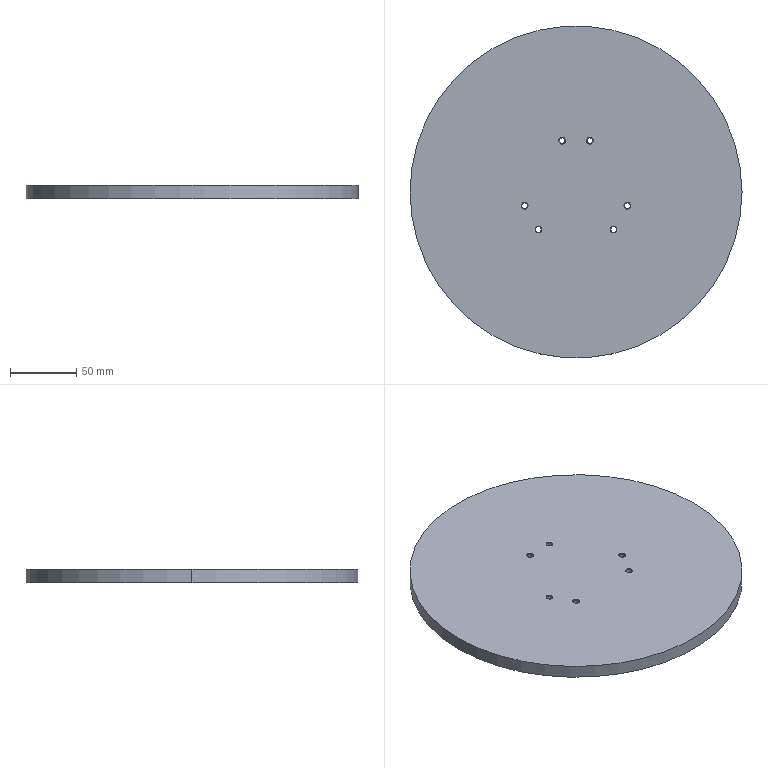Part | SolidWorks | features 3DProfileFeature 1, CirPattern 1, Extrusion 1, HoleWzd 1 | 1 solid | 28 faces | box 250 x 250 x 10 mm | volume 490035 mm3 | cylinder 14 | cone 12 | plane 2 | commonest cylinder face diameters 4.2 x12 250 x2
STEP:
#1=CARTESIAN_POINT('',(26.184,-28.284,9.575));
#2=VERTEX_POINT('',#1);
#3=CARTESIAN_POINT('',(30.384,-28.284,9.575));
#4=VERTEX_POINT('',#3);
#5=CARTESIAN_POINT('',(28.284,-28.284,9.575));
#6=DIRECTION('',(0.,0.,1.));
#7=DIRECTION('',(1.,0.,0.));
#8=AXIS2_PLACEMENT_3D('',#5,#6,#7);
#9=CIRCLE('',#8,2.1);
#10=EDGE_CURVE('',#2,#4,#9,.T.);
#11=ORIENTED_EDGE('',*,*,#10,.F.);
#12=CARTESIAN_POINT('',(25.759,-28.284,10.));
#13=VERTEX_POINT('',#12);
#14=CARTESIAN_POINT('',(25.759,-28.284,10.));
#15=DIRECTION('',(-0.7071,0.,0.7071));
#16=VECTOR('',#15,1000.);
#17=LINE('',#14,#16);
#18=EDGE_CURVE('',#2,#13,#17,.T.);
#19=ORIENTED_EDGE('',*,*,#18,.T.);
#20=CARTESIAN_POINT('',(30.809,-28.284,10.));
#21=VERTEX_POINT('',#20);
#22=CARTESIAN_POINT('',(28.284,-28.284,10.));
#23=DIRECTION('',(0.,0.,1.));
#24=DIRECTION('',(1.,0.,0.));
#25=AXIS2_PLACEMENT_3D('',#22,#23,#24);
#26=CIRCLE('',#25,2.525);
#27=EDGE_CURVE('',#13,#21,#26,.T.);
#28=ORIENTED_EDGE('',*,*,#27,.T.);
#29=CARTESIAN_POINT('',(30.809,-28.284,10.));
#30=DIRECTION('',(0.7071,0.,0.7071));
#31=VECTOR('',#30,1000.);
#32=LINE('',#29,#31);
#33=EDGE_CURVE('',#4,#21,#32,.T.);
#34=ORIENTED_EDGE('',*,*,#33,.F.);
#35=EDGE_LOOP('',(#11,#19,#28,#34));
#36=FACE_OUTER_BOUND('',#35,.T.);
#37=CARTESIAN_POINT('',(28.284,-28.284,10.));
#38=DIRECTION('',(0.,0.,1.));
#39=DIRECTION('',(1.,0.,0.));
#40=AXIS2_PLACEMENT_3D('',#37,#38,#39);
#41=CONICAL_SURFACE('',#40,2.525,0.7854);
#42=ADVANCED_FACE('',(#36),#41,.F.);
#43=CARTESIAN_POINT('',(26.184,-28.284,0.));
#44=VERTEX_POINT('',#43);
#45=CARTESIAN_POINT('',(30.384,-28.284,0.));
#46=VERTEX_POINT('',#45);
#47=CARTESIAN_POINT('',(28.284,-28.284,0.));
#48=DIRECTION('',(0.,0.,1.));
#49=DIRECTION('',(1.,0.,0.));
#50=AXIS2_PLACEMENT_3D('',#47,#48,#49);
#51=CIRCLE('',#50,2.1);
#52=EDGE_CURVE('',#44,#46,#51,.T.);
#53=ORIENTED_EDGE('',*,*,#52,.F.);
#54=CARTESIAN_POINT('',(26.184,-28.284,10.));
#55=DIRECTION('',(0.,0.,1.));
#56=VECTOR('',#55,1000.);
#57=LINE('',#54,#56);
#58=EDGE_CURVE('',#44,#2,#57,.T.);
#59=ORIENTED_EDGE('',*,*,#58,.T.);
#60=ORIENTED_EDGE('',*,*,#10,.T.);
#61=CARTESIAN_POINT('',(30.384,-28.284,10.));
#62=DIRECTION('',(0.,0.,1.));
#63=VECTOR('',#62,1000.);
#64=LINE('',#61,#63);
#65=EDGE_CURVE('',#46,#4,#64,.T.);
#66=ORIENTED_EDGE('',*,*,#65,.F.);
#67=EDGE_LOOP('',(#53,#59,#60,#66));
#68=FACE_OUTER_BOUND('',#67,.T.);
#69=CARTESIAN_POINT('',(28.284,-28.284,10.));
#70=DIRECTION('',(0.,0.,1.));
#71=DIRECTION('',(1.,0.,0.));
#72=AXIS2_PLACEMENT_3D('',#69,#70,#71);
#73=CYLINDRICAL_SURFACE('',#72,2.1);
#74=ADVANCED_FACE('',(#68),#73,.F.);
#75=CARTESIAN_POINT('',(36.537,-10.353,9.575));
#76=VERTEX_POINT('',#75);
#77=CARTESIAN_POINT('',(40.737,-10.353,9.575));
#78=VERTEX_POINT('',#77);
#79=CARTESIAN_POINT('',(38.637,-10.353,9.575));
#80=DIRECTION('',(0.,0.,1.));
#81=DIRECTION('',(1.,0.,0.));
#82=AXIS2_PLACEMENT_3D('',#79,#80,#81);
#83=CIRCLE('',#82,2.1);
#84=EDGE_CURVE('',#76,#78,#83,.T.);
#85=ORIENTED_EDGE('',*,*,#84,.F.);
#86=CARTESIAN_POINT('',(36.112,-10.353,10.));
#87=VERTEX_POINT('',#86);
#88=CARTESIAN_POINT('',(36.112,-10.353,10.));
#89=DIRECTION('',(-0.7071,0.,0.7071));
#90=VECTOR('',#89,1000.);
#91=LINE('',#88,#90);
#92=EDGE_CURVE('',#76,#87,#91,.T.);
#93=ORIENTED_EDGE('',*,*,#92,.T.);
#94=CARTESIAN_POINT('',(41.162,-10.353,10.));
#95=VERTEX_POINT('',#94);
#96=CARTESIAN_POINT('',(38.637,-10.353,10.));
#97=DIRECTION('',(0.,0.,1.));
#98=DIRECTION('',(1.,0.,0.));
#99=AXIS2_PLACEMENT_3D('',#96,#97,#98);
#100=CIRCLE('',#99,2.525);
#101=EDGE_CURVE('',#87,#95,#100,.T.);
#102=ORIENTED_EDGE('',*,*,#101,.T.);
#103=CARTESIAN_POINT('',(41.162,-10.353,10.));
#104=DIRECTION('',(0.7071,0.,0.7071));
#105=VECTOR('',#104,1000.);
#106=LINE('',#103,#105);
#107=EDGE_CURVE('',#78,#95,#106,.T.);
#108=ORIENTED_EDGE('',*,*,#107,.F.);
#109=EDGE_LOOP('',(#85,#93,#102,#108));
#110=FACE_OUTER_BOUND('',#109,.T.);
#111=CARTESIAN_POINT('',(38.637,-10.353,10.));
#112=DIRECTION('',(0.,0.,1.));
#113=DIRECTION('',(1.,0.,0.));
#114=AXIS2_PLACEMENT_3D('',#111,#112,#113);
#115=CONICAL_SURFACE('',#114,2.525,0.7854);
#116=ADVANCED_FACE('',(#110),#115,.F.);
#117=CARTESIAN_POINT('',(36.537,-10.353,0.));
#118=VERTEX_POINT('',#117);
#119=CARTESIAN_POINT('',(40.737,-10.353,0.));
#120=VERTEX_POINT('',#119);
#121=CARTESIAN_POINT('',(38.637,-10.353,0.));
#122=DIRECTION('',(0.,0.,1.));
#123=DIRECTION('',(1.,0.,0.));
#124=AXIS2_PLACEMENT_3D('',#121,#122,#123);
#125=CIRCLE('',#124,2.1);
#126=EDGE_CURVE('',#118,#120,#125,.T.);
#127=ORIENTED_EDGE('',*,*,#126,.F.);
#128=CARTESIAN_POINT('',(36.537,-10.353,10.));
#129=DIRECTION('',(0.,0.,1.));
#130=VECTOR('',#129,1000.);
#131=LINE('',#128,#130);
#132=EDGE_CURVE('',#118,#76,#131,.T.);
#133=ORIENTED_EDGE('',*,*,#132,.T.);
#134=ORIENTED_EDGE('',*,*,#84,.T.);
#135=CARTESIAN_POINT('',(40.737,-10.353,10.));
#136=DIRECTION('',(0.,0.,1.));
#137=VECTOR('',#136,1000.);
#138=LINE('',#135,#137);
#139=EDGE_CURVE('',#120,#78,#138,.T.);
#140=ORIENTED_EDGE('',*,*,#139,.F.);
#141=EDGE_LOOP('',(#127,#133,#134,#140));
#142=FACE_OUTER_BOUND('',#141,.T.);
#143=CARTESIAN_POINT('',(38.637,-10.353,10.));
#144=DIRECTION('',(0.,0.,1.));
#145=DIRECTION('',(1.,0.,0.));
#146=AXIS2_PLACEMENT_3D('',#143,#144,#145);
#147=CYLINDRICAL_SURFACE('',#146,2.1);
#148=ADVANCED_FACE('',(#142),#147,.F.);
#149=CARTESIAN_POINT('',(-40.737,-10.353,9.575));
#150=VERTEX_POINT('',#149);
#151=CARTESIAN_POINT('',(-36.537,-10.353,9.575));
#152=VERTEX_POINT('',#151);
#153=CARTESIAN_POINT('',(-38.637,-10.353,9.575));
#154=DIRECTION('',(0.,0.,1.));
#155=DIRECTION('',(1.,0.,0.));
#156=AXIS2_PLACEMENT_3D('',#153,#154,#155);
#157=CIRCLE('',#156,2.1);
#158=EDGE_CURVE('',#150,#152,#157,.T.);
#159=ORIENTED_EDGE('',*,*,#158,.F.);
#160=CARTESIAN_POINT('',(-41.162,-10.353,10.));
#161=VERTEX_POINT('',#160);
#162=CARTESIAN_POINT('',(-41.162,-10.353,10.));
#163=DIRECTION('',(-0.7071,0.,0.7071));
#164=VECTOR('',#163,1000.);
#165=LINE('',#162,#164);
#166=EDGE_CURVE('',#150,#161,#165,.T.);
#167=ORIENTED_EDGE('',*,*,#166,.T.);
#168=CARTESIAN_POINT('',(-36.112,-10.353,10.));
#169=VERTEX_POINT('',#168);
#170=CARTESIAN_POINT('',(-38.637,-10.353,10.));
#171=DIRECTION('',(0.,0.,1.));
#172=DIRECTION('',(1.,0.,0.));
#173=AXIS2_PLACEMENT_3D('',#170,#171,#172);
#174=CIRCLE('',#173,2.525);
#175=EDGE_CURVE('',#161,#169,#174,.T.);
#176=ORIENTED_EDGE('',*,*,#175,.T.);
#177=CARTESIAN_POINT('',(-36.112,-10.353,10.));
#178=DIRECTION('',(0.7071,0.,0.7071));
#179=VECTOR('',#178,1000.);
#180=LINE('',#177,#179);
#181=EDGE_CURVE('',#152,#169,#180,.T.);
#182=ORIENTED_EDGE('',*,*,#181,.F.);
#183=EDGE_LOOP('',(#159,#167,#176,#182));
#184=FACE_OUTER_BOUND('',#183,.T.);
#185=CARTESIAN_POINT('',(-38.637,-10.353,10.));
#186=DIRECTION('',(0.,0.,1.));
#187=DIRECTION('',(1.,0.,0.));
#188=AXIS2_PLACEMENT_3D('',#185,#186,#187);
#189=CONICAL_SURFACE('',#188,2.525,0.7854);
#190=ADVANCED_FACE('',(#184),#189,.F.);
#191=CARTESIAN_POINT('',(-40.737,-10.353,0.));
#192=VERTEX_POINT('',#191);
#193=CARTESIAN_POINT('',(-36.537,-10.353,0.));
#194=VERTEX_POINT('',#193);
#195=CARTESIAN_POINT('',(-38.637,-10.353,0.));
#196=DIRECTION('',(0.,0.,1.));
#197=DIRECTION('',(1.,0.,0.));
#198=AXIS2_PLACEMENT_3D('',#195,#196,#197);
#199=CIRCLE('',#198,2.1);
#200=EDGE_CURVE('',#192,#194,#199,.T.);
#201=ORIENTED_EDGE('',*,*,#200,.F.);
#202=CARTESIAN_POINT('',(-40.737,-10.353,10.));
#203=DIRECTION('',(0.,0.,1.));
#204=VECTOR('',#203,1000.);
#205=LINE('',#202,#204);
#206=EDGE_CURVE('',#192,#150,#205,.T.);
#207=ORIENTED_EDGE('',*,*,#206,.T.);
#208=ORIENTED_EDGE('',*,*,#158,.T.);
#209=CARTESIAN_POINT('',(-36.537,-10.353,10.));
#210=DIRECTION('',(0.,0.,1.));
#211=VECTOR('',#210,1000.);
#212=LINE('',#209,#211);
#213=EDGE_CURVE('',#194,#152,#212,.T.);
#214=ORIENTED_EDGE('',*,*,#213,.F.);
#215=EDGE_LOOP('',(#201,#207,#208,#214));
#216=FACE_OUTER_BOUND('',#215,.T.);
#217=CARTESIAN_POINT('',(-38.637,-10.353,10.));
#218=DIRECTION('',(0.,0.,1.));
#219=DIRECTION('',(1.,0.,0.));
#220=AXIS2_PLACEMENT_3D('',#217,#218,#219);
#221=CYLINDRICAL_SURFACE('',#220,2.1);
#222=ADVANCED_FACE('',(#216),#221,.F.);
#223=CARTESIAN_POINT('',(-30.384,-28.284,9.575));
#224=VERTEX_POINT('',#223);
#225=CARTESIAN_POINT('',(-26.184,-28.284,9.575));
#226=VERTEX_POINT('',#225);
#227=CARTESIAN_POINT('',(-28.284,-28.284,9.575));
#228=DIRECTION('',(0.,0.,1.));
#229=DIRECTION('',(1.,0.,0.));
#230=AXIS2_PLACEMENT_3D('',#227,#228,#229);
#231=CIRCLE('',#230,2.1);
#232=EDGE_CURVE('',#224,#226,#231,.T.);
#233=ORIENTED_EDGE('',*,*,#232,.F.);
#234=CARTESIAN_POINT('',(-30.809,-28.284,10.));
#235=VERTEX_POINT('',#234);
#236=CARTESIAN_POINT('',(-30.809,-28.284,10.));
#237=DIRECTION('',(-0.7071,0.,0.7071));
#238=VECTOR('',#237,1000.);
#239=LINE('',#236,#238);
#240=EDGE_CURVE('',#224,#235,#239,.T.);
#241=ORIENTED_EDGE('',*,*,#240,.T.);
#242=CARTESIAN_POINT('',(-25.759,-28.284,10.));
#243=VERTEX_POINT('',#242);
#244=CARTESIAN_POINT('',(-28.284,-28.284,10.));
#245=DIRECTION('',(0.,0.,1.));
#246=DIRECTION('',(1.,0.,0.));
#247=AXIS2_PLACEMENT_3D('',#244,#245,#246);
#248=CIRCLE('',#247,2.525);
#249=EDGE_CURVE('',#235,#243,#248,.T.);
#250=ORIENTED_EDGE('',*,*,#249,.T.);
#251=CARTESIAN_POINT('',(-25.759,-28.284,10.));
#252=DIRECTION('',(0.7071,0.,0.7071));
#253=VECTOR('',#252,1000.);
#254=LINE('',#251,#253);
#255=EDGE_CURVE('',#226,#243,#254,.T.);
#256=ORIENTED_EDGE('',*,*,#255,.F.);
#257=EDGE_LOOP('',(#233,#241,#250,#256));
#258=FACE_OUTER_BOUND('',#257,.T.);
#259=CARTESIAN_POINT('',(-28.284,-28.284,10.));
#260=DIRECTION('',(0.,0.,1.));
#261=DIRECTION('',(1.,0.,0.));
#262=AXIS2_PLACEMENT_3D('',#259,#260,#261);
#263=CONICAL_SURFACE('',#262,2.525,0.7854);
#264=ADVANCED_FACE('',(#258),#263,.F.);
#265=CARTESIAN_POINT('',(-30.384,-28.284,0.));
#266=VERTEX_POINT('',#265);
#267=CARTESIAN_POINT('',(-26.184,-28.284,0.));
#268=VERTEX_POINT('',#267);
#269=CARTESIAN_POINT('',(-28.284,-28.284,0.));
#270=DIRECTION('',(0.,0.,1.));
#271=DIRECTION('',(1.,0.,0.));
#272=AXIS2_PLACEMENT_3D('',#269,#270,#271);
#273=CIRCLE('',#272,2.1);
#274=EDGE_CURVE('',#266,#268,#273,.T.);
#275=ORIENTED_EDGE('',*,*,#274,.F.);
#276=CARTESIAN_POINT('',(-30.384,-28.284,10.));
#277=DIRECTION('',(0.,0.,1.));
#278=VECTOR('',#277,1000.);
#279=LINE('',#276,#278);
#280=EDGE_CURVE('',#266,#224,#279,.T.);
#281=ORIENTED_EDGE('',*,*,#280,.T.);
#282=ORIENTED_EDGE('',*,*,#232,.T.);
#283=CARTESIAN_POINT('',(-26.184,-28.284,10.));
#284=DIRECTION('',(0.,0.,1.));
#285=VECTOR('',#284,1000.);
#286=LINE('',#283,#285);
#287=EDGE_CURVE('',#268,#226,#286,.T.);
#288=ORIENTED_EDGE('',*,*,#287,.F.);
#289=EDGE_LOOP('',(#275,#281,#282,#288));
#290=FACE_OUTER_BOUND('',#289,.T.);
#291=CARTESIAN_POINT('',(-28.284,-28.284,10.));
#292=DIRECTION('',(0.,0.,1.));
#293=DIRECTION('',(1.,0.,0.));
#294=AXIS2_PLACEMENT_3D('',#291,#292,#293);
#295=CYLINDRICAL_SURFACE('',#294,2.1);
#296=ADVANCED_FACE('',(#290),#295,.F.);
#297=CARTESIAN_POINT('',(8.253,38.637,9.575));
#298=VERTEX_POINT('',#297);
#299=CARTESIAN_POINT('',(12.453,38.637,9.575));
#300=VERTEX_POINT('',#299);
#301=CARTESIAN_POINT('',(10.353,38.637,9.575));
#302=DIRECTION('',(0.,0.,1.));
#303=DIRECTION('',(1.,0.,0.));
#304=AXIS2_PLACEMENT_3D('',#301,#302,#303);
#305=CIRCLE('',#304,2.1);
#306=EDGE_CURVE('',#298,#300,#305,.T.);
#307=ORIENTED_EDGE('',*,*,#306,.F.);
#308=CARTESIAN_POINT('',(7.828,38.637,10.));
#309=VERTEX_POINT('',#308);
#310=CARTESIAN_POINT('',(7.828,38.637,10.));
#311=DIRECTION('',(-0.7071,0.,0.7071));
#312=VECTOR('',#311,1000.);
#313=LINE('',#310,#312);
#314=EDGE_CURVE('',#298,#309,#313,.T.);
#315=ORIENTED_EDGE('',*,*,#314,.T.);
#316=CARTESIAN_POINT('',(12.878,38.637,10.));
#317=VERTEX_POINT('',#316);
#318=CARTESIAN_POINT('',(10.353,38.637,10.));
#319=DIRECTION('',(0.,0.,1.));
#320=DIRECTION('',(1.,0.,0.));
#321=AXIS2_PLACEMENT_3D('',#318,#319,#320);
#322=CIRCLE('',#321,2.525);
#323=EDGE_CURVE('',#309,#317,#322,.T.);
#324=ORIENTED_EDGE('',*,*,#323,.T.);
#325=CARTESIAN_POINT('',(12.878,38.637,10.));
#326=DIRECTION('',(0.7071,0.,0.7071));
#327=VECTOR('',#326,1000.);
#328=LINE('',#325,#327);
#329=EDGE_CURVE('',#300,#317,#328,.T.);
#330=ORIENTED_EDGE('',*,*,#329,.F.);
#331=EDGE_LOOP('',(#307,#315,#324,#330));
#332=FACE_OUTER_BOUND('',#331,.T.);
#333=CARTESIAN_POINT('',(10.353,38.637,10.));
#334=DIRECTION('',(0.,0.,1.));
#335=DIRECTION('',(1.,0.,0.));
#336=AXIS2_PLACEMENT_3D('',#333,#334,#335);
#337=CONICAL_SURFACE('',#336,2.525,0.7854);
#338=ADVANCED_FACE('',(#332),#337,.F.);
#339=CARTESIAN_POINT('',(8.253,38.637,0.));
#340=VERTEX_POINT('',#339);
#341=CARTESIAN_POINT('',(12.453,38.637,0.));
#342=VERTEX_POINT('',#341);
#343=CARTESIAN_POINT('',(10.353,38.637,0.));
#344=DIRECTION('',(0.,0.,1.));
#345=DIRECTION('',(1.,0.,0.));
#346=AXIS2_PLACEMENT_3D('',#343,#344,#345);
#347=CIRCLE('',#346,2.1);
#348=EDGE_CURVE('',#340,#342,#347,.T.);
#349=ORIENTED_EDGE('',*,*,#348,.F.);
#350=CARTESIAN_POINT('',(8.253,38.637,10.));
#351=DIRECTION('',(0.,0.,1.));
#352=VECTOR('',#351,1000.);
#353=LINE('',#350,#352);
#354=EDGE_CURVE('',#340,#298,#353,.T.);
#355=ORIENTED_EDGE('',*,*,#354,.T.);
#356=ORIENTED_EDGE('',*,*,#306,.T.);
#357=CARTESIAN_POINT('',(12.453,38.637,10.));
#358=DIRECTION('',(0.,0.,1.));
#359=VECTOR('',#358,1000.);
#360=LINE('',#357,#359);
#361=EDGE_CURVE('',#342,#300,#360,.T.);
#362=ORIENTED_EDGE('',*,*,#361,.F.);
#363=EDGE_LOOP('',(#349,#355,#356,#362));
#364=FACE_OUTER_BOUND('',#363,.T.);
#365=CARTESIAN_POINT('',(10.353,38.637,10.));
#366=DIRECTION('',(0.,0.,1.));
#367=DIRECTION('',(1.,0.,0.));
#368=AXIS2_PLACEMENT_3D('',#365,#366,#367);
#369=CYLINDRICAL_SURFACE('',#368,2.1);
#370=ADVANCED_FACE('',(#364),#369,.F.);
#371=CARTESIAN_POINT('',(-12.453,38.637,9.575));
#372=VERTEX_POINT('',#371);
#373=CARTESIAN_POINT('',(-8.253,38.637,9.575));
#374=VERTEX_POINT('',#373);
#375=CARTESIAN_POINT('',(-10.353,38.637,9.575));
#376=DIRECTION('',(0.,0.,1.));
#377=DIRECTION('',(1.,0.,0.));
#378=AXIS2_PLACEMENT_3D('',#375,#376,#377);
#379=CIRCLE('',#378,2.1);
#380=EDGE_CURVE('',#372,#374,#379,.T.);
#381=ORIENTED_EDGE('',*,*,#380,.F.);
#382=CARTESIAN_POINT('',(-12.878,38.637,10.));
#383=VERTEX_POINT('',#382);
#384=CARTESIAN_POINT('',(-12.878,38.637,10.));
#385=DIRECTION('',(-0.7071,0.,0.7071));
#386=VECTOR('',#385,1000.);
#387=LINE('',#384,#386);
#388=EDGE_CURVE('',#372,#383,#387,.T.);
#389=ORIENTED_EDGE('',*,*,#388,.T.);
#390=CARTESIAN_POINT('',(-7.828,38.637,10.));
#391=VERTEX_POINT('',#390);
#392=CARTESIAN_POINT('',(-10.353,38.637,10.));
#393=DIRECTION('',(0.,0.,1.));
#394=DIRECTION('',(1.,0.,0.));
#395=AXIS2_PLACEMENT_3D('',#392,#393,#394);
#396=CIRCLE('',#395,2.525);
#397=EDGE_CURVE('',#383,#391,#396,.T.);
#398=ORIENTED_EDGE('',*,*,#397,.T.);
#399=CARTESIAN_POINT('',(-7.828,38.637,10.));
#400=DIRECTION('',(0.7071,0.,0.7071));
#401=VECTOR('',#400,1000.);
#402=LINE('',#399,#401);
#403=EDGE_CURVE('',#374,#391,#402,.T.);
#404=ORIENTED_EDGE('',*,*,#403,.F.);
#405=EDGE_LOOP('',(#381,#389,#398,#404));
#406=FACE_OUTER_BOUND('',#405,.T.);
#407=CARTESIAN_POINT('',(-10.353,38.637,10.));
#408=DIRECTION('',(0.,0.,1.));
#409=DIRECTION('',(1.,0.,0.));
#410=AXIS2_PLACEMENT_3D('',#407,#408,#409);
#411=CONICAL_SURFACE('',#410,2.525,0.7854);
#412=ADVANCED_FACE('',(#406),#411,.F.);
#413=CARTESIAN_POINT('',(-12.453,38.637,0.));
#414=VERTEX_POINT('',#413);
#415=CARTESIAN_POINT('',(-8.253,38.637,0.));
#416=VERTEX_POINT('',#415);
#417=CARTESIAN_POINT('',(-10.353,38.637,0.));
#418=DIRECTION('',(0.,0.,1.));
#419=DIRECTION('',(1.,0.,0.));
#420=AXIS2_PLACEMENT_3D('',#417,#418,#419);
#421=CIRCLE('',#420,2.1);
#422=EDGE_CURVE('',#414,#416,#421,.T.);
#423=ORIENTED_EDGE('',*,*,#422,.F.);
#424=CARTESIAN_POINT('',(-12.453,38.637,10.));
#425=DIRECTION('',(0.,0.,1.));
#426=VECTOR('',#425,1000.);
#427=LINE('',#424,#426);
#428=EDGE_CURVE('',#414,#372,#427,.T.);
#429=ORIENTED_EDGE('',*,*,#428,.T.);
#430=ORIENTED_EDGE('',*,*,#380,.T.);
#431=CARTESIAN_POINT('',(-8.253,38.637,10.));
#432=DIRECTION('',(0.,0.,1.));
#433=VECTOR('',#432,1000.);
#434=LINE('',#431,#433);
#435=EDGE_CURVE('',#416,#374,#434,.T.);
#436=ORIENTED_EDGE('',*,*,#435,.F.);
#437=EDGE_LOOP('',(#423,#429,#430,#436));
#438=FACE_OUTER_BOUND('',#437,.T.);
#439=CARTESIAN_POINT('',(-10.353,38.637,10.));
#440=DIRECTION('',(0.,0.,1.));
#441=DIRECTION('',(1.,0.,0.));
#442=AXIS2_PLACEMENT_3D('',#439,#440,#441);
#443=CYLINDRICAL_SURFACE('',#442,2.1);
#444=ADVANCED_FACE('',(#438),#443,.F.);
#445=CARTESIAN_POINT('',(125.,0.,10.));
#446=VERTEX_POINT('',#445);
#447=CARTESIAN_POINT('',(-125.,0.,10.));
#448=VERTEX_POINT('',#447);
#449=CARTESIAN_POINT('',(0.,0.,10.));
#450=DIRECTION('',(0.,0.,1.));
#451=DIRECTION('',(1.,0.,0.));
#452=AXIS2_PLACEMENT_3D('',#449,#450,#451);
#453=CIRCLE('',#452,125.);
#454=EDGE_CURVE('',#446,#448,#453,.T.);
#455=ORIENTED_EDGE('',*,*,#454,.F.);
#456=CARTESIAN_POINT('',(125.,0.,0.));
#457=VERTEX_POINT('',#456);
#458=CARTESIAN_POINT('',(125.,0.,10.));
#459=DIRECTION('',(0.,0.,-1.));
#460=VECTOR('',#459,1000.);
#461=LINE('',#458,#460);
#462=EDGE_CURVE('',#446,#457,#461,.T.);
#463=ORIENTED_EDGE('',*,*,#462,.T.);
#464=CARTESIAN_POINT('',(-125.,0.,0.));
#465=VERTEX_POINT('',#464);
#466=CARTESIAN_POINT('',(0.,0.,0.));
#467=DIRECTION('',(0.,0.,1.));
#468=DIRECTION('',(1.,0.,0.));
#469=AXIS2_PLACEMENT_3D('',#466,#467,#468);
#470=CIRCLE('',#469,125.);
#471=EDGE_CURVE('',#457,#465,#470,.T.);
#472=ORIENTED_EDGE('',*,*,#471,.T.);
#473=CARTESIAN_POINT('',(-125.,0.,10.));
#474=DIRECTION('',(0.,0.,-1.));
#475=VECTOR('',#474,1000.);
#476=LINE('',#473,#475);
#477=EDGE_CURVE('',#448,#465,#476,.T.);
#478=ORIENTED_EDGE('',*,*,#477,.F.);
#479=EDGE_LOOP('',(#455,#463,#472,#478));
#480=FACE_OUTER_BOUND('',#479,.T.);
#481=CARTESIAN_POINT('',(0.,0.,10.));
#482=DIRECTION('',(0.,0.,-1.));
#483=DIRECTION('',(-1.,0.,0.));
#484=AXIS2_PLACEMENT_3D('',#481,#482,#483);
#485=CYLINDRICAL_SURFACE('',#484,125.);
#486=ADVANCED_FACE('',(#480),#485,.T.);
#487=ORIENTED_EDGE('',*,*,#462,.F.);
#488=CARTESIAN_POINT('',(0.,0.,10.));
#489=DIRECTION('',(0.,0.,1.));
#490=DIRECTION('',(1.,0.,0.));
#491=AXIS2_PLACEMENT_3D('',#488,#489,#490);
#492=CIRCLE('',#491,125.);
#493=EDGE_CURVE('',#448,#446,#492,.T.);
#494=ORIENTED_EDGE('',*,*,#493,.F.);
#495=ORIENTED_EDGE('',*,*,#477,.T.);
#496=CARTESIAN_POINT('',(0.,0.,0.));
#497=DIRECTION('',(0.,0.,1.));
#498=DIRECTION('',(1.,0.,0.));
#499=AXIS2_PLACEMENT_3D('',#496,#497,#498);
#500=CIRCLE('',#499,125.);
#501=EDGE_CURVE('',#465,#457,#500,.T.);
#502=ORIENTED_EDGE('',*,*,#501,.T.);
#503=EDGE_LOOP('',(#487,#494,#495,#502));
#504=FACE_OUTER_BOUND('',#503,.T.);
#505=CARTESIAN_POINT('',(0.,0.,10.));
#506=DIRECTION('',(0.,0.,-1.));
#507=DIRECTION('',(-1.,0.,0.));
#508=AXIS2_PLACEMENT_3D('',#505,#506,#507);
#509=CYLINDRICAL_SURFACE('',#508,125.);
#510=ADVANCED_FACE('',(#504),#509,.T.);
#511=CARTESIAN_POINT('',(28.284,-28.284,10.));
#512=DIRECTION('',(0.,0.,1.));
#513=DIRECTION('',(1.,0.,0.));
#514=AXIS2_PLACEMENT_3D('',#511,#512,#513);
#515=CIRCLE('',#514,2.525);
#516=EDGE_CURVE('',#21,#13,#515,.T.);
#517=ORIENTED_EDGE('',*,*,#516,.F.);
#518=ORIENTED_EDGE('',*,*,#27,.F.);
#519=EDGE_LOOP('',(#517,#518));
#520=FACE_BOUND('',#519,.T.);
#521=CARTESIAN_POINT('',(38.637,-10.353,10.));
#522=DIRECTION('',(0.,0.,1.));
#523=DIRECTION('',(1.,0.,0.));
#524=AXIS2_PLACEMENT_3D('',#521,#522,#523);
#525=CIRCLE('',#524,2.525);
#526=EDGE_CURVE('',#95,#87,#525,.T.);
#527=ORIENTED_EDGE('',*,*,#526,.F.);
#528=ORIENTED_EDGE('',*,*,#101,.F.);
#529=EDGE_LOOP('',(#527,#528));
#530=FACE_BOUND('',#529,.T.);
#531=CARTESIAN_POINT('',(-38.637,-10.353,10.));
#532=DIRECTION('',(0.,0.,1.));
#533=DIRECTION('',(1.,0.,0.));
#534=AXIS2_PLACEMENT_3D('',#531,#532,#533);
#535=CIRCLE('',#534,2.525);
#536=EDGE_CURVE('',#169,#161,#535,.T.);
#537=ORIENTED_EDGE('',*,*,#536,.F.);
#538=ORIENTED_EDGE('',*,*,#175,.F.);
#539=EDGE_LOOP('',(#537,#538));
#540=FACE_BOUND('',#539,.T.);
#541=CARTESIAN_POINT('',(-28.284,-28.284,10.));
#542=DIRECTION('',(0.,0.,1.));
#543=DIRECTION('',(1.,0.,0.));
#544=AXIS2_PLACEMENT_3D('',#541,#542,#543);
#545=CIRCLE('',#544,2.525);
#546=EDGE_CURVE('',#243,#235,#545,.T.);
#547=ORIENTED_EDGE('',*,*,#546,.F.);
#548=ORIENTED_EDGE('',*,*,#249,.F.);
#549=EDGE_LOOP('',(#547,#548));
#550=FACE_BOUND('',#549,.T.);
#551=CARTESIAN_POINT('',(10.353,38.637,10.));
#552=DIRECTION('',(0.,0.,1.));
#553=DIRECTION('',(1.,0.,0.));
#554=AXIS2_PLACEMENT_3D('',#551,#552,#553);
#555=CIRCLE('',#554,2.525);
#556=EDGE_CURVE('',#317,#309,#555,.T.);
#557=ORIENTED_EDGE('',*,*,#556,.F.);
#558=ORIENTED_EDGE('',*,*,#323,.F.);
#559=EDGE_LOOP('',(#557,#558));
#560=FACE_BOUND('',#559,.T.);
#561=CARTESIAN_POINT('',(-10.353,38.637,10.));
#562=DIRECTION('',(0.,0.,1.));
#563=DIRECTION('',(1.,0.,0.));
#564=AXIS2_PLACEMENT_3D('',#561,#562,#563);
#565=CIRCLE('',#564,2.525);
#566=EDGE_CURVE('',#391,#383,#565,.T.);
#567=ORIENTED_EDGE('',*,*,#566,.F.);
#568=ORIENTED_EDGE('',*,*,#397,.F.);
#569=EDGE_LOOP('',(#567,#568));
#570=FACE_BOUND('',#569,.T.);
#571=ORIENTED_EDGE('',*,*,#493,.T.);
#572=ORIENTED_EDGE('',*,*,#454,.T.);
#573=EDGE_LOOP('',(#571,#572));
#574=FACE_OUTER_BOUND('',#573,.T.);
#575=CARTESIAN_POINT('',(0.,0.,10.));
#576=DIRECTION('',(0.,0.,1.));
#577=DIRECTION('',(1.,0.,0.));
#578=AXIS2_PLACEMENT_3D('',#575,#576,#577);
#579=PLANE('',#578);
#580=ADVANCED_FACE('',(#520,#530,#540,#550,#560,#570,#574),#579,.T.);
#581=CARTESIAN_POINT('',(28.284,-28.284,0.));
#582=DIRECTION('',(0.,0.,1.));
#583=DIRECTION('',(1.,0.,0.));
#584=AXIS2_PLACEMENT_3D('',#581,#582,#583);
#585=CIRCLE('',#584,2.1);
#586=EDGE_CURVE('',#46,#44,#585,.T.);
#587=ORIENTED_EDGE('',*,*,#586,.T.);
#588=ORIENTED_EDGE('',*,*,#52,.T.);
#589=EDGE_LOOP('',(#587,#588));
#590=FACE_BOUND('',#589,.T.);
#591=CARTESIAN_POINT('',(38.637,-10.353,0.));
#592=DIRECTION('',(0.,0.,1.));
#593=DIRECTION('',(1.,0.,0.));
#594=AXIS2_PLACEMENT_3D('',#591,#592,#593);
#595=CIRCLE('',#594,2.1);
#596=EDGE_CURVE('',#120,#118,#595,.T.);
#597=ORIENTED_EDGE('',*,*,#596,.T.);
#598=ORIENTED_EDGE('',*,*,#126,.T.);
#599=EDGE_LOOP('',(#597,#598));
#600=FACE_BOUND('',#599,.T.);
#601=CARTESIAN_POINT('',(-38.637,-10.353,0.));
#602=DIRECTION('',(0.,0.,1.));
#603=DIRECTION('',(1.,0.,0.));
#604=AXIS2_PLACEMENT_3D('',#601,#602,#603);
#605=CIRCLE('',#604,2.1);
#606=EDGE_CURVE('',#194,#192,#605,.T.);
#607=ORIENTED_EDGE('',*,*,#606,.T.);
#608=ORIENTED_EDGE('',*,*,#200,.T.);
#609=EDGE_LOOP('',(#607,#608));
#610=FACE_BOUND('',#609,.T.);
#611=CARTESIAN_POINT('',(-28.284,-28.284,0.));
#612=DIRECTION('',(0.,0.,1.));
#613=DIRECTION('',(1.,0.,0.));
#614=AXIS2_PLACEMENT_3D('',#611,#612,#613);
#615=CIRCLE('',#614,2.1);
#616=EDGE_CURVE('',#268,#266,#615,.T.);
#617=ORIENTED_EDGE('',*,*,#616,.T.);
#618=ORIENTED_EDGE('',*,*,#274,.T.);
#619=EDGE_LOOP('',(#617,#618));
#620=FACE_BOUND('',#619,.T.);
#621=CARTESIAN_POINT('',(10.353,38.637,0.));
#622=DIRECTION('',(0.,0.,1.));
#623=DIRECTION('',(1.,0.,0.));
#624=AXIS2_PLACEMENT_3D('',#621,#622,#623);
#625=CIRCLE('',#624,2.1);
#626=EDGE_CURVE('',#342,#340,#625,.T.);
#627=ORIENTED_EDGE('',*,*,#626,.T.);
#628=ORIENTED_EDGE('',*,*,#348,.T.);
#629=EDGE_LOOP('',(#627,#628));
#630=FACE_BOUND('',#629,.T.);
#631=CARTESIAN_POINT('',(-10.353,38.637,0.));
#632=DIRECTION('',(0.,0.,1.));
#633=DIRECTION('',(1.,0.,0.));
#634=AXIS2_PLACEMENT_3D('',#631,#632,#633);
#635=CIRCLE('',#634,2.1);
#636=EDGE_CURVE('',#416,#414,#635,.T.);
#637=ORIENTED_EDGE('',*,*,#636,.T.);
#638=ORIENTED_EDGE('',*,*,#422,.T.);
#639=EDGE_LOOP('',(#637,#638));
#640=FACE_BOUND('',#639,.T.);
#641=ORIENTED_EDGE('',*,*,#501,.F.);
#642=ORIENTED_EDGE('',*,*,#471,.F.);
#643=EDGE_LOOP('',(#641,#642));
#644=FACE_OUTER_BOUND('',#643,.T.);
#645=CARTESIAN_POINT('',(0.,0.,0.));
#646=DIRECTION('',(0.,0.,1.));
#647=DIRECTION('',(1.,0.,0.));
#648=AXIS2_PLACEMENT_3D('',#645,#646,#647);
#649=PLANE('',#648);
#650=ADVANCED_FACE('',(#590,#600,#610,#620,#630,#640,#644),#649,.F.);
#651=ORIENTED_EDGE('',*,*,#428,.F.);
#652=ORIENTED_EDGE('',*,*,#636,.F.);
#653=ORIENTED_EDGE('',*,*,#435,.T.);
#654=CARTESIAN_POINT('',(-10.353,38.637,9.575));
#655=DIRECTION('',(0.,0.,1.));
#656=DIRECTION('',(1.,0.,0.));
#657=AXIS2_PLACEMENT_3D('',#654,#655,#656);
#658=CIRCLE('',#657,2.1);
#659=EDGE_CURVE('',#374,#372,#658,.T.);
#660=ORIENTED_EDGE('',*,*,#659,.T.);
#661=EDGE_LOOP('',(#651,#652,#653,#660));
#662=FACE_OUTER_BOUND('',#661,.T.);
#663=CARTESIAN_POINT('',(-10.353,38.637,10.));
#664=DIRECTION('',(0.,0.,1.));
#665=DIRECTION('',(1.,0.,0.));
#666=AXIS2_PLACEMENT_3D('',#663,#664,#665);
#667=CYLINDRICAL_SURFACE('',#666,2.1);
#668=ADVANCED_FACE('',(#662),#667,.F.);
#669=ORIENTED_EDGE('',*,*,#388,.F.);
#670=ORIENTED_EDGE('',*,*,#659,.F.);
#671=ORIENTED_EDGE('',*,*,#403,.T.);
#672=ORIENTED_EDGE('',*,*,#566,.T.);
#673=EDGE_LOOP('',(#669,#670,#671,#672));
#674=FACE_OUTER_BOUND('',#673,.T.);
#675=CARTESIAN_POINT('',(-10.353,38.637,10.));
#676=DIRECTION('',(0.,0.,1.));
#677=DIRECTION('',(1.,0.,0.));
#678=AXIS2_PLACEMENT_3D('',#675,#676,#677);
#679=CONICAL_SURFACE('',#678,2.525,0.7854);
#680=ADVANCED_FACE('',(#674),#679,.F.);
#681=ORIENTED_EDGE('',*,*,#354,.F.);
#682=ORIENTED_EDGE('',*,*,#626,.F.);
#683=ORIENTED_EDGE('',*,*,#361,.T.);
#684=CARTESIAN_POINT('',(10.353,38.637,9.575));
#685=DIRECTION('',(0.,0.,1.));
#686=DIRECTION('',(1.,0.,0.));
#687=AXIS2_PLACEMENT_3D('',#684,#685,#686);
#688=CIRCLE('',#687,2.1);
#689=EDGE_CURVE('',#300,#298,#688,.T.);
#690=ORIENTED_EDGE('',*,*,#689,.T.);
#691=EDGE_LOOP('',(#681,#682,#683,#690));
#692=FACE_OUTER_BOUND('',#691,.T.);
#693=CARTESIAN_POINT('',(10.353,38.637,10.));
#694=DIRECTION('',(0.,0.,1.));
#695=DIRECTION('',(1.,0.,0.));
#696=AXIS2_PLACEMENT_3D('',#693,#694,#695);
#697=CYLINDRICAL_SURFACE('',#696,2.1);
#698=ADVANCED_FACE('',(#692),#697,.F.);
#699=ORIENTED_EDGE('',*,*,#314,.F.);
#700=ORIENTED_EDGE('',*,*,#689,.F.);
#701=ORIENTED_EDGE('',*,*,#329,.T.);
#702=ORIENTED_EDGE('',*,*,#556,.T.);
#703=EDGE_LOOP('',(#699,#700,#701,#702));
#704=FACE_OUTER_BOUND('',#703,.T.);
#705=CARTESIAN_POINT('',(10.353,38.637,10.));
#706=DIRECTION('',(0.,0.,1.));
#707=DIRECTION('',(1.,0.,0.));
#708=AXIS2_PLACEMENT_3D('',#705,#706,#707);
#709=CONICAL_SURFACE('',#708,2.525,0.7854);
#710=ADVANCED_FACE('',(#704),#709,.F.);
#711=ORIENTED_EDGE('',*,*,#280,.F.);
#712=ORIENTED_EDGE('',*,*,#616,.F.);
#713=ORIENTED_EDGE('',*,*,#287,.T.);
#714=CARTESIAN_POINT('',(-28.284,-28.284,9.575));
#715=DIRECTION('',(0.,0.,1.));
#716=DIRECTION('',(1.,0.,0.));
#717=AXIS2_PLACEMENT_3D('',#714,#715,#716);
#718=CIRCLE('',#717,2.1);
#719=EDGE_CURVE('',#226,#224,#718,.T.);
#720=ORIENTED_EDGE('',*,*,#719,.T.);
#721=EDGE_LOOP('',(#711,#712,#713,#720));
#722=FACE_OUTER_BOUND('',#721,.T.);
#723=CARTESIAN_POINT('',(-28.284,-28.284,10.));
#724=DIRECTION('',(0.,0.,1.));
#725=DIRECTION('',(1.,0.,0.));
#726=AXIS2_PLACEMENT_3D('',#723,#724,#725);
#727=CYLINDRICAL_SURFACE('',#726,2.1);
#728=ADVANCED_FACE('',(#722),#727,.F.);
#729=ORIENTED_EDGE('',*,*,#240,.F.);
#730=ORIENTED_EDGE('',*,*,#719,.F.);
#731=ORIENTED_EDGE('',*,*,#255,.T.);
#732=ORIENTED_EDGE('',*,*,#546,.T.);
#733=EDGE_LOOP('',(#729,#730,#731,#732));
#734=FACE_OUTER_BOUND('',#733,.T.);
#735=CARTESIAN_POINT('',(-28.284,-28.284,10.));
#736=DIRECTION('',(0.,0.,1.));
#737=DIRECTION('',(1.,0.,0.));
#738=AXIS2_PLACEMENT_3D('',#735,#736,#737);
#739=CONICAL_SURFACE('',#738,2.525,0.7854);
#740=ADVANCED_FACE('',(#734),#739,.F.);
#741=ORIENTED_EDGE('',*,*,#206,.F.);
#742=ORIENTED_EDGE('',*,*,#606,.F.);
#743=ORIENTED_EDGE('',*,*,#213,.T.);
#744=CARTESIAN_POINT('',(-38.637,-10.353,9.575));
#745=DIRECTION('',(0.,0.,1.));
#746=DIRECTION('',(1.,0.,0.));
#747=AXIS2_PLACEMENT_3D('',#744,#745,#746);
#748=CIRCLE('',#747,2.1);
#749=EDGE_CURVE('',#152,#150,#748,.T.);
#750=ORIENTED_EDGE('',*,*,#749,.T.);
#751=EDGE_LOOP('',(#741,#742,#743,#750));
#752=FACE_OUTER_BOUND('',#751,.T.);
#753=CARTESIAN_POINT('',(-38.637,-10.353,10.));
#754=DIRECTION('',(0.,0.,1.));
#755=DIRECTION('',(1.,0.,0.));
#756=AXIS2_PLACEMENT_3D('',#753,#754,#755);
#757=CYLINDRICAL_SURFACE('',#756,2.1);
#758=ADVANCED_FACE('',(#752),#757,.F.);
#759=ORIENTED_EDGE('',*,*,#166,.F.);
#760=ORIENTED_EDGE('',*,*,#749,.F.);
#761=ORIENTED_EDGE('',*,*,#181,.T.);
#762=ORIENTED_EDGE('',*,*,#536,.T.);
#763=EDGE_LOOP('',(#759,#760,#761,#762));
#764=FACE_OUTER_BOUND('',#763,.T.);
#765=CARTESIAN_POINT('',(-38.637,-10.353,10.));
#766=DIRECTION('',(0.,0.,1.));
#767=DIRECTION('',(1.,0.,0.));
#768=AXIS2_PLACEMENT_3D('',#765,#766,#767);
#769=CONICAL_SURFACE('',#768,2.525,0.7854);
#770=ADVANCED_FACE('',(#764),#769,.F.);
#771=ORIENTED_EDGE('',*,*,#132,.F.);
#772=ORIENTED_EDGE('',*,*,#596,.F.);
#773=ORIENTED_EDGE('',*,*,#139,.T.);
#774=CARTESIAN_POINT('',(38.637,-10.353,9.575));
#775=DIRECTION('',(0.,0.,1.));
#776=DIRECTION('',(1.,0.,0.));
#777=AXIS2_PLACEMENT_3D('',#774,#775,#776);
#778=CIRCLE('',#777,2.1);
#779=EDGE_CURVE('',#78,#76,#778,.T.);
#780=ORIENTED_EDGE('',*,*,#779,.T.);
#781=EDGE_LOOP('',(#771,#772,#773,#780));
#782=FACE_OUTER_BOUND('',#781,.T.);
#783=CARTESIAN_POINT('',(38.637,-10.353,10.));
#784=DIRECTION('',(0.,0.,1.));
#785=DIRECTION('',(1.,0.,0.));
#786=AXIS2_PLACEMENT_3D('',#783,#784,#785);
#787=CYLINDRICAL_SURFACE('',#786,2.1);
#788=ADVANCED_FACE('',(#782),#787,.F.);
#789=ORIENTED_EDGE('',*,*,#92,.F.);
#790=ORIENTED_EDGE('',*,*,#779,.F.);
#791=ORIENTED_EDGE('',*,*,#107,.T.);
#792=ORIENTED_EDGE('',*,*,#526,.T.);
#793=EDGE_LOOP('',(#789,#790,#791,#792));
#794=FACE_OUTER_BOUND('',#793,.T.);
#795=CARTESIAN_POINT('',(38.637,-10.353,10.));
#796=DIRECTION('',(0.,0.,1.));
#797=DIRECTION('',(1.,0.,0.));
#798=AXIS2_PLACEMENT_3D('',#795,#796,#797);
#799=CONICAL_SURFACE('',#798,2.525,0.7854);
#800=ADVANCED_FACE('',(#794),#799,.F.);
#801=ORIENTED_EDGE('',*,*,#58,.F.);
#802=ORIENTED_EDGE('',*,*,#586,.F.);
#803=ORIENTED_EDGE('',*,*,#65,.T.);
#804=CARTESIAN_POINT('',(28.284,-28.284,9.575));
#805=DIRECTION('',(0.,0.,1.));
#806=DIRECTION('',(1.,0.,0.));
#807=AXIS2_PLACEMENT_3D('',#804,#805,#806);
#808=CIRCLE('',#807,2.1);
#809=EDGE_CURVE('',#4,#2,#808,.T.);
#810=ORIENTED_EDGE('',*,*,#809,.T.);
#811=EDGE_LOOP('',(#801,#802,#803,#810));
#812=FACE_OUTER_BOUND('',#811,.T.);
#813=CARTESIAN_POINT('',(28.284,-28.284,10.));
#814=DIRECTION('',(0.,0.,1.));
#815=DIRECTION('',(1.,0.,0.));
#816=AXIS2_PLACEMENT_3D('',#813,#814,#815);
#817=CYLINDRICAL_SURFACE('',#816,2.1);
#818=ADVANCED_FACE('',(#812),#817,.F.);
#819=ORIENTED_EDGE('',*,*,#18,.F.);
#820=ORIENTED_EDGE('',*,*,#809,.F.);
#821=ORIENTED_EDGE('',*,*,#33,.T.);
#822=ORIENTED_EDGE('',*,*,#516,.T.);
#823=EDGE_LOOP('',(#819,#820,#821,#822));
#824=FACE_OUTER_BOUND('',#823,.T.);
#825=CARTESIAN_POINT('',(28.284,-28.284,10.));
#826=DIRECTION('',(0.,0.,1.));
#827=DIRECTION('',(1.,0.,0.));
#828=AXIS2_PLACEMENT_3D('',#825,#826,#827);
#829=CONICAL_SURFACE('',#828,2.525,0.7854);
#830=ADVANCED_FACE('',(#824),#829,.F.);
#831=CLOSED_SHELL('',(#42,#74,#116,#148,#190,#222,#264,#296,#338,#370,#412,#444,#486,#510,#580,#650,#668,#680,#698,#710,#728,#740,#758,#770,#788,#800,#818,#830));
#832=MANIFOLD_SOLID_BREP('',#831);
#833=CARTESIAN_POINT('',(0.,0.,0.));
#834=DIRECTION('',(0.,0.,1.));
#835=DIRECTION('',(1.,0.,0.));
#836=AXIS2_PLACEMENT_3D('',#833,#834,#835);
#837=(LENGTH_UNIT()NAMED_UNIT(*)SI_UNIT(.MILLI.,.METRE.));
#838=UNCERTAINTY_MEASURE_WITH_UNIT(LENGTH_MEASURE(0.00001),#837,'','');
#839=(NAMED_UNIT(*)PLANE_ANGLE_UNIT()SI_UNIT($,.RADIAN.));
#840=(NAMED_UNIT(*)SI_UNIT($,.STERADIAN.)SOLID_ANGLE_UNIT());
#841=(GEOMETRIC_REPRESENTATION_CONTEXT(3)GLOBAL_UNCERTAINTY_ASSIGNED_CONTEXT((#838))GLOBAL_UNIT_ASSIGNED_CONTEXT((#837,#839,#840))REPRESENTATION_CONTEXT('',''));
#842=ADVANCED_BREP_SHAPE_REPRESENTATION('',(#832,#836),#841);